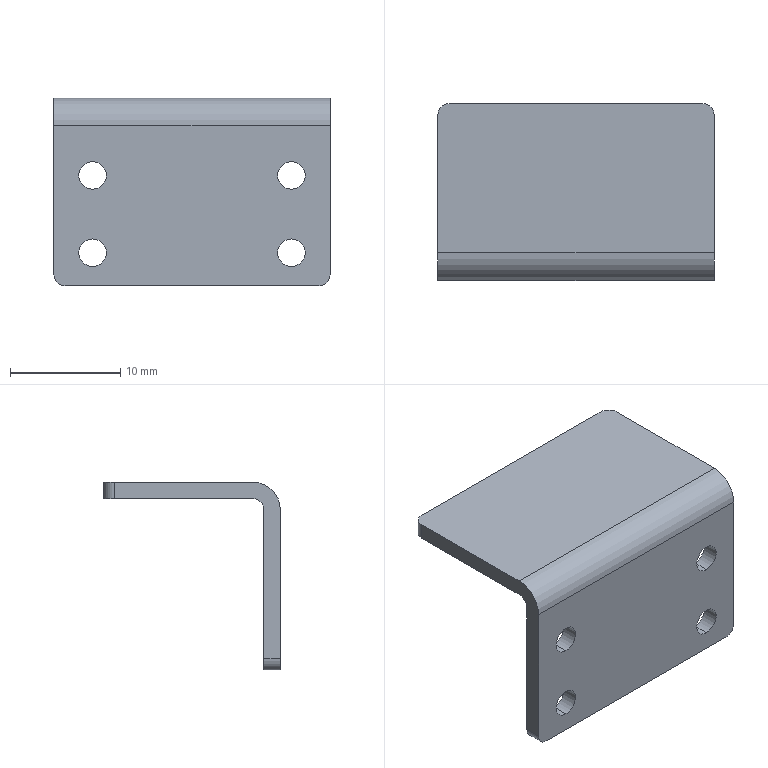Part | SolidWorks | features BaseBody 1 | 1 solid | 22 faces | box 25 x 16 x 17 mm | volume 1122 mm3 | cylinder 14 | plane 8 | commonest cylinder face diameters 2.5 x8 2 x5 5 x1
STEP:
#1=CARTESIAN_POINT('',(100.5,20.,-73.25));
#2=VERTEX_POINT('',#1);
#3=CARTESIAN_POINT('',(100.5,20.,-75.75));
#4=VERTEX_POINT('',#3);
#5=CARTESIAN_POINT('',(100.5,20.,-74.5));
#6=DIRECTION('',(0.,-1.,0.));
#7=DIRECTION('',(0.,0.,1.));
#8=AXIS2_PLACEMENT_3D('',#5,#6,#7);
#9=CIRCLE('',#8,1.25);
#10=EDGE_CURVE('',#2,#4,#9,.T.);
#11=ORIENTED_EDGE('',*,*,#10,.T.);
#12=CARTESIAN_POINT('',(100.5,21.5,-75.75));
#13=VERTEX_POINT('',#12);
#14=CARTESIAN_POINT('',(100.5,46.5,-75.75));
#15=DIRECTION('',(0.,1.,0.));
#16=VECTOR('',#15,1000.);
#17=LINE('',#14,#16);
#18=EDGE_CURVE('',#4,#13,#17,.T.);
#19=ORIENTED_EDGE('',*,*,#18,.T.);
#20=CARTESIAN_POINT('',(100.5,21.5,-73.25));
#21=VERTEX_POINT('',#20);
#22=CARTESIAN_POINT('',(100.5,21.5,-74.5));
#23=DIRECTION('',(0.,-1.,0.));
#24=DIRECTION('',(0.,0.,1.));
#25=AXIS2_PLACEMENT_3D('',#22,#23,#24);
#26=CIRCLE('',#25,1.25);
#27=EDGE_CURVE('',#21,#13,#26,.T.);
#28=ORIENTED_EDGE('',*,*,#27,.F.);
#29=CARTESIAN_POINT('',(100.5,46.5,-73.25));
#30=DIRECTION('',(0.,1.,0.));
#31=VECTOR('',#30,1000.);
#32=LINE('',#29,#31);
#33=EDGE_CURVE('',#2,#21,#32,.T.);
#34=ORIENTED_EDGE('',*,*,#33,.F.);
#35=EDGE_LOOP('',(#11,#19,#28,#34));
#36=FACE_OUTER_BOUND('',#35,.T.);
#37=CARTESIAN_POINT('',(100.5,46.5,-74.5));
#38=DIRECTION('',(0.,1.,0.));
#39=DIRECTION('',(0.,0.,1.));
#40=AXIS2_PLACEMENT_3D('',#37,#38,#39);
#41=CYLINDRICAL_SURFACE('',#40,1.25);
#42=ADVANCED_FACE('',(#36),#41,.F.);
#43=CARTESIAN_POINT('',(118.5,20.,-80.25));
#44=VERTEX_POINT('',#43);
#45=CARTESIAN_POINT('',(118.5,20.,-82.75));
#46=VERTEX_POINT('',#45);
#47=CARTESIAN_POINT('',(118.5,20.,-81.5));
#48=DIRECTION('',(0.,-1.,0.));
#49=DIRECTION('',(0.,0.,1.));
#50=AXIS2_PLACEMENT_3D('',#47,#48,#49);
#51=CIRCLE('',#50,1.25);
#52=EDGE_CURVE('',#44,#46,#51,.T.);
#53=ORIENTED_EDGE('',*,*,#52,.T.);
#54=CARTESIAN_POINT('',(118.5,21.5,-82.75));
#55=VERTEX_POINT('',#54);
#56=CARTESIAN_POINT('',(118.5,46.5,-82.75));
#57=DIRECTION('',(0.,1.,0.));
#58=VECTOR('',#57,1000.);
#59=LINE('',#56,#58);
#60=EDGE_CURVE('',#46,#55,#59,.T.);
#61=ORIENTED_EDGE('',*,*,#60,.T.);
#62=CARTESIAN_POINT('',(118.5,21.5,-80.25));
#63=VERTEX_POINT('',#62);
#64=CARTESIAN_POINT('',(118.5,21.5,-81.5));
#65=DIRECTION('',(0.,-1.,0.));
#66=DIRECTION('',(0.,0.,1.));
#67=AXIS2_PLACEMENT_3D('',#64,#65,#66);
#68=CIRCLE('',#67,1.25);
#69=EDGE_CURVE('',#63,#55,#68,.T.);
#70=ORIENTED_EDGE('',*,*,#69,.F.);
#71=CARTESIAN_POINT('',(118.5,46.5,-80.25));
#72=DIRECTION('',(0.,1.,0.));
#73=VECTOR('',#72,1000.);
#74=LINE('',#71,#73);
#75=EDGE_CURVE('',#44,#63,#74,.T.);
#76=ORIENTED_EDGE('',*,*,#75,.F.);
#77=EDGE_LOOP('',(#53,#61,#70,#76));
#78=FACE_OUTER_BOUND('',#77,.T.);
#79=CARTESIAN_POINT('',(118.5,46.5,-81.5));
#80=DIRECTION('',(0.,1.,0.));
#81=DIRECTION('',(0.,0.,1.));
#82=AXIS2_PLACEMENT_3D('',#79,#80,#81);
#83=CYLINDRICAL_SURFACE('',#82,1.25);
#84=ADVANCED_FACE('',(#78),#83,.F.);
#85=CARTESIAN_POINT('',(100.5,20.,-80.25));
#86=VERTEX_POINT('',#85);
#87=CARTESIAN_POINT('',(100.5,20.,-82.75));
#88=VERTEX_POINT('',#87);
#89=CARTESIAN_POINT('',(100.5,20.,-81.5));
#90=DIRECTION('',(0.,-1.,0.));
#91=DIRECTION('',(0.,0.,1.));
#92=AXIS2_PLACEMENT_3D('',#89,#90,#91);
#93=CIRCLE('',#92,1.25);
#94=EDGE_CURVE('',#86,#88,#93,.T.);
#95=ORIENTED_EDGE('',*,*,#94,.T.);
#96=CARTESIAN_POINT('',(100.5,21.5,-82.75));
#97=VERTEX_POINT('',#96);
#98=CARTESIAN_POINT('',(100.5,46.5,-82.75));
#99=DIRECTION('',(0.,1.,0.));
#100=VECTOR('',#99,1000.);
#101=LINE('',#98,#100);
#102=EDGE_CURVE('',#88,#97,#101,.T.);
#103=ORIENTED_EDGE('',*,*,#102,.T.);
#104=CARTESIAN_POINT('',(100.5,21.5,-80.25));
#105=VERTEX_POINT('',#104);
#106=CARTESIAN_POINT('',(100.5,21.5,-81.5));
#107=DIRECTION('',(0.,-1.,0.));
#108=DIRECTION('',(0.,0.,1.));
#109=AXIS2_PLACEMENT_3D('',#106,#107,#108);
#110=CIRCLE('',#109,1.25);
#111=EDGE_CURVE('',#105,#97,#110,.T.);
#112=ORIENTED_EDGE('',*,*,#111,.F.);
#113=CARTESIAN_POINT('',(100.5,46.5,-80.25));
#114=DIRECTION('',(0.,1.,0.));
#115=VECTOR('',#114,1000.);
#116=LINE('',#113,#115);
#117=EDGE_CURVE('',#86,#105,#116,.T.);
#118=ORIENTED_EDGE('',*,*,#117,.F.);
#119=EDGE_LOOP('',(#95,#103,#112,#118));
#120=FACE_OUTER_BOUND('',#119,.T.);
#121=CARTESIAN_POINT('',(100.5,46.5,-81.5));
#122=DIRECTION('',(0.,1.,0.));
#123=DIRECTION('',(0.,0.,1.));
#124=AXIS2_PLACEMENT_3D('',#121,#122,#123);
#125=CYLINDRICAL_SURFACE('',#124,1.25);
#126=ADVANCED_FACE('',(#120),#125,.F.);
#127=CARTESIAN_POINT('',(118.5,20.,-73.25));
#128=VERTEX_POINT('',#127);
#129=CARTESIAN_POINT('',(118.5,20.,-75.75));
#130=VERTEX_POINT('',#129);
#131=CARTESIAN_POINT('',(118.5,20.,-74.5));
#132=DIRECTION('',(0.,-1.,0.));
#133=DIRECTION('',(0.,0.,1.));
#134=AXIS2_PLACEMENT_3D('',#131,#132,#133);
#135=CIRCLE('',#134,1.25);
#136=EDGE_CURVE('',#128,#130,#135,.T.);
#137=ORIENTED_EDGE('',*,*,#136,.T.);
#138=CARTESIAN_POINT('',(118.5,21.5,-75.75));
#139=VERTEX_POINT('',#138);
#140=CARTESIAN_POINT('',(118.5,46.5,-75.75));
#141=DIRECTION('',(0.,1.,0.));
#142=VECTOR('',#141,1000.);
#143=LINE('',#140,#142);
#144=EDGE_CURVE('',#130,#139,#143,.T.);
#145=ORIENTED_EDGE('',*,*,#144,.T.);
#146=CARTESIAN_POINT('',(118.5,21.5,-73.25));
#147=VERTEX_POINT('',#146);
#148=CARTESIAN_POINT('',(118.5,21.5,-74.5));
#149=DIRECTION('',(0.,-1.,0.));
#150=DIRECTION('',(0.,0.,1.));
#151=AXIS2_PLACEMENT_3D('',#148,#149,#150);
#152=CIRCLE('',#151,1.25);
#153=EDGE_CURVE('',#147,#139,#152,.T.);
#154=ORIENTED_EDGE('',*,*,#153,.F.);
#155=CARTESIAN_POINT('',(118.5,46.5,-73.25));
#156=DIRECTION('',(0.,1.,0.));
#157=VECTOR('',#156,1000.);
#158=LINE('',#155,#157);
#159=EDGE_CURVE('',#128,#147,#158,.T.);
#160=ORIENTED_EDGE('',*,*,#159,.F.);
#161=EDGE_LOOP('',(#137,#145,#154,#160));
#162=FACE_OUTER_BOUND('',#161,.T.);
#163=CARTESIAN_POINT('',(118.5,46.5,-74.5));
#164=DIRECTION('',(0.,1.,0.));
#165=DIRECTION('',(0.,0.,1.));
#166=AXIS2_PLACEMENT_3D('',#163,#164,#165);
#167=CYLINDRICAL_SURFACE('',#166,1.25);
#168=ADVANCED_FACE('',(#162),#167,.F.);
#169=CARTESIAN_POINT('',(122.,20.,-83.5));
#170=VERTEX_POINT('',#169);
#171=CARTESIAN_POINT('',(121.,20.,-84.5));
#172=VERTEX_POINT('',#171);
#173=CARTESIAN_POINT('',(121.,20.,-83.5));
#174=DIRECTION('',(0.,1.,0.));
#175=DIRECTION('',(0.,0.,1.));
#176=AXIS2_PLACEMENT_3D('',#173,#174,#175);
#177=CIRCLE('',#176,1.);
#178=EDGE_CURVE('',#170,#172,#177,.T.);
#179=ORIENTED_EDGE('',*,*,#178,.F.);
#180=CARTESIAN_POINT('',(122.,20.,-70.));
#181=VERTEX_POINT('',#180);
#182=CARTESIAN_POINT('',(122.,20.,-70.));
#183=DIRECTION('',(0.,0.,-1.));
#184=VECTOR('',#183,1000.);
#185=LINE('',#182,#184);
#186=EDGE_CURVE('',#181,#170,#185,.T.);
#187=ORIENTED_EDGE('',*,*,#186,.F.);
#188=CARTESIAN_POINT('',(97.,20.,-70.));
#189=VERTEX_POINT('',#188);
#190=CARTESIAN_POINT('',(122.,20.,-70.));
#191=DIRECTION('',(1.,0.,0.));
#192=VECTOR('',#191,1000.);
#193=LINE('',#190,#192);
#194=EDGE_CURVE('',#189,#181,#193,.T.);
#195=ORIENTED_EDGE('',*,*,#194,.F.);
#196=CARTESIAN_POINT('',(97.,20.,-83.5));
#197=VERTEX_POINT('',#196);
#198=CARTESIAN_POINT('',(97.,20.,-70.));
#199=DIRECTION('',(0.,0.,1.));
#200=VECTOR('',#199,1000.);
#201=LINE('',#198,#200);
#202=EDGE_CURVE('',#197,#189,#201,.T.);
#203=ORIENTED_EDGE('',*,*,#202,.F.);
#204=CARTESIAN_POINT('',(98.,20.,-84.5));
#205=VERTEX_POINT('',#204);
#206=CARTESIAN_POINT('',(98.,20.,-83.5));
#207=DIRECTION('',(0.,1.,0.));
#208=DIRECTION('',(0.,0.,-1.));
#209=AXIS2_PLACEMENT_3D('',#206,#207,#208);
#210=CIRCLE('',#209,1.);
#211=EDGE_CURVE('',#205,#197,#210,.T.);
#212=ORIENTED_EDGE('',*,*,#211,.F.);
#213=CARTESIAN_POINT('',(122.,20.,-84.5));
#214=DIRECTION('',(-1.,0.,0.));
#215=VECTOR('',#214,1000.);
#216=LINE('',#213,#215);
#217=EDGE_CURVE('',#172,#205,#216,.T.);
#218=ORIENTED_EDGE('',*,*,#217,.F.);
#219=EDGE_LOOP('',(#179,#187,#195,#203,#212,#218));
#220=FACE_OUTER_BOUND('',#219,.T.);
#221=ORIENTED_EDGE('',*,*,#10,.F.);
#222=CARTESIAN_POINT('',(100.5,20.,-74.5));
#223=DIRECTION('',(0.,-1.,0.));
#224=DIRECTION('',(0.,0.,1.));
#225=AXIS2_PLACEMENT_3D('',#222,#223,#224);
#226=CIRCLE('',#225,1.25);
#227=EDGE_CURVE('',#4,#2,#226,.T.);
#228=ORIENTED_EDGE('',*,*,#227,.F.);
#229=EDGE_LOOP('',(#221,#228));
#230=FACE_BOUND('',#229,.T.);
#231=ORIENTED_EDGE('',*,*,#52,.F.);
#232=CARTESIAN_POINT('',(118.5,20.,-81.5));
#233=DIRECTION('',(0.,-1.,0.));
#234=DIRECTION('',(0.,0.,1.));
#235=AXIS2_PLACEMENT_3D('',#232,#233,#234);
#236=CIRCLE('',#235,1.25);
#237=EDGE_CURVE('',#46,#44,#236,.T.);
#238=ORIENTED_EDGE('',*,*,#237,.F.);
#239=EDGE_LOOP('',(#231,#238));
#240=FACE_BOUND('',#239,.T.);
#241=ORIENTED_EDGE('',*,*,#94,.F.);
#242=CARTESIAN_POINT('',(100.5,20.,-81.5));
#243=DIRECTION('',(0.,-1.,0.));
#244=DIRECTION('',(0.,0.,1.));
#245=AXIS2_PLACEMENT_3D('',#242,#243,#244);
#246=CIRCLE('',#245,1.25);
#247=EDGE_CURVE('',#88,#86,#246,.T.);
#248=ORIENTED_EDGE('',*,*,#247,.F.);
#249=EDGE_LOOP('',(#241,#248));
#250=FACE_BOUND('',#249,.T.);
#251=ORIENTED_EDGE('',*,*,#136,.F.);
#252=CARTESIAN_POINT('',(118.5,20.,-74.5));
#253=DIRECTION('',(0.,-1.,0.));
#254=DIRECTION('',(0.,0.,1.));
#255=AXIS2_PLACEMENT_3D('',#252,#253,#254);
#256=CIRCLE('',#255,1.25);
#257=EDGE_CURVE('',#130,#128,#256,.T.);
#258=ORIENTED_EDGE('',*,*,#257,.F.);
#259=EDGE_LOOP('',(#251,#258));
#260=FACE_BOUND('',#259,.T.);
#261=CARTESIAN_POINT('',(122.,20.,-70.));
#262=DIRECTION('',(0.,1.,0.));
#263=DIRECTION('',(0.,0.,1.));
#264=AXIS2_PLACEMENT_3D('',#261,#262,#263);
#265=PLANE('',#264);
#266=ADVANCED_FACE('',(#220,#230,#240,#250,#260),#265,.F.);
#267=CARTESIAN_POINT('',(121.,21.5,-84.5));
#268=VERTEX_POINT('',#267);
#269=CARTESIAN_POINT('',(121.,20.,-84.5));
#270=DIRECTION('',(0.,1.,0.));
#271=VECTOR('',#270,1000.);
#272=LINE('',#269,#271);
#273=EDGE_CURVE('',#172,#268,#272,.T.);
#274=ORIENTED_EDGE('',*,*,#273,.F.);
#275=ORIENTED_EDGE('',*,*,#217,.T.);
#276=CARTESIAN_POINT('',(98.,21.5,-84.5));
#277=VERTEX_POINT('',#276);
#278=CARTESIAN_POINT('',(98.,20.,-84.5));
#279=DIRECTION('',(0.,-1.,0.));
#280=VECTOR('',#279,1000.);
#281=LINE('',#278,#280);
#282=EDGE_CURVE('',#277,#205,#281,.T.);
#283=ORIENTED_EDGE('',*,*,#282,.F.);
#284=CARTESIAN_POINT('',(122.,21.5,-84.5));
#285=DIRECTION('',(-1.,0.,0.));
#286=VECTOR('',#285,1000.);
#287=LINE('',#284,#286);
#288=EDGE_CURVE('',#268,#277,#287,.T.);
#289=ORIENTED_EDGE('',*,*,#288,.F.);
#290=EDGE_LOOP('',(#274,#275,#283,#289));
#291=FACE_OUTER_BOUND('',#290,.T.);
#292=CARTESIAN_POINT('',(122.,20.,-84.5));
#293=DIRECTION('',(0.,0.,1.));
#294=DIRECTION('',(1.,0.,0.));
#295=AXIS2_PLACEMENT_3D('',#292,#293,#294);
#296=PLANE('',#295);
#297=ADVANCED_FACE('',(#291),#296,.F.);
#298=CARTESIAN_POINT('',(122.,21.5,-83.5));
#299=VERTEX_POINT('',#298);
#300=CARTESIAN_POINT('',(121.,21.5,-83.5));
#301=DIRECTION('',(0.,-1.,0.));
#302=DIRECTION('',(0.,0.,1.));
#303=AXIS2_PLACEMENT_3D('',#300,#301,#302);
#304=CIRCLE('',#303,1.);
#305=EDGE_CURVE('',#268,#299,#304,.T.);
#306=ORIENTED_EDGE('',*,*,#305,.T.);
#307=CARTESIAN_POINT('',(122.,22.5,-83.5));
#308=DIRECTION('',(0.,-1.,0.));
#309=VECTOR('',#308,1000.);
#310=LINE('',#307,#309);
#311=EDGE_CURVE('',#299,#170,#310,.T.);
#312=ORIENTED_EDGE('',*,*,#311,.T.);
#313=ORIENTED_EDGE('',*,*,#178,.T.);
#314=ORIENTED_EDGE('',*,*,#273,.T.);
#315=EDGE_LOOP('',(#306,#312,#313,#314));
#316=FACE_OUTER_BOUND('',#315,.T.);
#317=CARTESIAN_POINT('',(121.,22.5,-83.5));
#318=DIRECTION('',(0.,1.,0.));
#319=DIRECTION('',(0.,0.,1.));
#320=AXIS2_PLACEMENT_3D('',#317,#318,#319);
#321=CYLINDRICAL_SURFACE('',#320,1.);
#322=ADVANCED_FACE('',(#316),#321,.T.);
#323=CARTESIAN_POINT('',(122.,35.,-67.5));
#324=VERTEX_POINT('',#323);
#325=CARTESIAN_POINT('',(122.,22.5,-67.5));
#326=VERTEX_POINT('',#325);
#327=CARTESIAN_POINT('',(122.,22.5,-67.5));
#328=DIRECTION('',(0.,-1.,0.));
#329=VECTOR('',#328,1000.);
#330=LINE('',#327,#329);
#331=EDGE_CURVE('',#324,#326,#330,.T.);
#332=ORIENTED_EDGE('',*,*,#331,.T.);
#333=CARTESIAN_POINT('',(122.,22.5,-70.));
#334=DIRECTION('',(1.,0.,0.));
#335=DIRECTION('',(0.,0.,-1.));
#336=AXIS2_PLACEMENT_3D('',#333,#334,#335);
#337=CIRCLE('',#336,2.5);
#338=EDGE_CURVE('',#326,#181,#337,.T.);
#339=ORIENTED_EDGE('',*,*,#338,.T.);
#340=ORIENTED_EDGE('',*,*,#186,.T.);
#341=ORIENTED_EDGE('',*,*,#311,.F.);
#342=CARTESIAN_POINT('',(122.,21.5,-70.));
#343=VERTEX_POINT('',#342);
#344=CARTESIAN_POINT('',(122.,21.5,-70.));
#345=DIRECTION('',(0.,0.,1.));
#346=VECTOR('',#345,1000.);
#347=LINE('',#344,#346);
#348=EDGE_CURVE('',#299,#343,#347,.T.);
#349=ORIENTED_EDGE('',*,*,#348,.T.);
#350=CARTESIAN_POINT('',(122.,22.5,-69.));
#351=VERTEX_POINT('',#350);
#352=CARTESIAN_POINT('',(122.,22.5,-70.));
#353=DIRECTION('',(-1.,0.,0.));
#354=DIRECTION('',(0.,0.,-1.));
#355=AXIS2_PLACEMENT_3D('',#352,#353,#354);
#356=CIRCLE('',#355,1.);
#357=EDGE_CURVE('',#343,#351,#356,.T.);
#358=ORIENTED_EDGE('',*,*,#357,.T.);
#359=CARTESIAN_POINT('',(122.,35.,-69.));
#360=VERTEX_POINT('',#359);
#361=CARTESIAN_POINT('',(122.,22.5,-69.));
#362=DIRECTION('',(0.,1.,0.));
#363=VECTOR('',#362,1000.);
#364=LINE('',#361,#363);
#365=EDGE_CURVE('',#351,#360,#364,.T.);
#366=ORIENTED_EDGE('',*,*,#365,.T.);
#367=CARTESIAN_POINT('',(122.,35.,-70.));
#368=DIRECTION('',(0.,0.,1.));
#369=VECTOR('',#368,1000.);
#370=LINE('',#367,#369);
#371=EDGE_CURVE('',#360,#324,#370,.T.);
#372=ORIENTED_EDGE('',*,*,#371,.T.);
#373=EDGE_LOOP('',(#332,#339,#340,#341,#349,#358,#366,#372));
#374=FACE_OUTER_BOUND('',#373,.T.);
#375=CARTESIAN_POINT('',(122.,22.5,-70.));
#376=DIRECTION('',(1.,0.,0.));
#377=DIRECTION('',(0.,0.,-1.));
#378=AXIS2_PLACEMENT_3D('',#375,#376,#377);
#379=PLANE('',#378);
#380=ADVANCED_FACE('',(#374),#379,.T.);
#381=ORIENTED_EDGE('',*,*,#338,.F.);
#382=CARTESIAN_POINT('',(97.,22.5,-67.5));
#383=VERTEX_POINT('',#382);
#384=CARTESIAN_POINT('',(122.,22.5,-67.5));
#385=DIRECTION('',(-1.,0.,0.));
#386=VECTOR('',#385,1000.);
#387=LINE('',#384,#386);
#388=EDGE_CURVE('',#326,#383,#387,.T.);
#389=ORIENTED_EDGE('',*,*,#388,.T.);
#390=CARTESIAN_POINT('',(97.,22.5,-70.));
#391=DIRECTION('',(1.,0.,0.));
#392=DIRECTION('',(0.,0.,-1.));
#393=AXIS2_PLACEMENT_3D('',#390,#391,#392);
#394=CIRCLE('',#393,2.5);
#395=EDGE_CURVE('',#383,#189,#394,.T.);
#396=ORIENTED_EDGE('',*,*,#395,.T.);
#397=ORIENTED_EDGE('',*,*,#194,.T.);
#398=EDGE_LOOP('',(#381,#389,#396,#397));
#399=FACE_OUTER_BOUND('',#398,.T.);
#400=CARTESIAN_POINT('',(122.,22.5,-70.));
#401=DIRECTION('',(1.,0.,0.));
#402=DIRECTION('',(0.,0.,-1.));
#403=AXIS2_PLACEMENT_3D('',#400,#401,#402);
#404=CYLINDRICAL_SURFACE('',#403,2.5);
#405=ADVANCED_FACE('',(#399),#404,.T.);
#406=CARTESIAN_POINT('',(97.,21.5,-83.5));
#407=VERTEX_POINT('',#406);
#408=CARTESIAN_POINT('',(97.,22.5,-83.5));
#409=DIRECTION('',(0.,1.,0.));
#410=VECTOR('',#409,1000.);
#411=LINE('',#408,#410);
#412=EDGE_CURVE('',#197,#407,#411,.T.);
#413=ORIENTED_EDGE('',*,*,#412,.F.);
#414=ORIENTED_EDGE('',*,*,#202,.T.);
#415=ORIENTED_EDGE('',*,*,#395,.F.);
#416=CARTESIAN_POINT('',(97.,35.,-67.5));
#417=VERTEX_POINT('',#416);
#418=CARTESIAN_POINT('',(97.,22.5,-67.5));
#419=DIRECTION('',(0.,-1.,0.));
#420=VECTOR('',#419,1000.);
#421=LINE('',#418,#420);
#422=EDGE_CURVE('',#417,#383,#421,.T.);
#423=ORIENTED_EDGE('',*,*,#422,.F.);
#424=CARTESIAN_POINT('',(97.,35.,-69.));
#425=VERTEX_POINT('',#424);
#426=CARTESIAN_POINT('',(97.,35.,-70.));
#427=DIRECTION('',(0.,0.,1.));
#428=VECTOR('',#427,1000.);
#429=LINE('',#426,#428);
#430=EDGE_CURVE('',#425,#417,#429,.T.);
#431=ORIENTED_EDGE('',*,*,#430,.F.);
#432=CARTESIAN_POINT('',(97.,22.5,-69.));
#433=VERTEX_POINT('',#432);
#434=CARTESIAN_POINT('',(97.,22.5,-69.));
#435=DIRECTION('',(0.,1.,0.));
#436=VECTOR('',#435,1000.);
#437=LINE('',#434,#436);
#438=EDGE_CURVE('',#433,#425,#437,.T.);
#439=ORIENTED_EDGE('',*,*,#438,.F.);
#440=CARTESIAN_POINT('',(97.,21.5,-70.));
#441=VERTEX_POINT('',#440);
#442=CARTESIAN_POINT('',(97.,22.5,-70.));
#443=DIRECTION('',(1.,0.,0.));
#444=DIRECTION('',(0.,0.,-1.));
#445=AXIS2_PLACEMENT_3D('',#442,#443,#444);
#446=CIRCLE('',#445,1.);
#447=EDGE_CURVE('',#433,#441,#446,.T.);
#448=ORIENTED_EDGE('',*,*,#447,.T.);
#449=CARTESIAN_POINT('',(97.,21.5,-70.));
#450=DIRECTION('',(0.,0.,1.));
#451=VECTOR('',#450,1000.);
#452=LINE('',#449,#451);
#453=EDGE_CURVE('',#407,#441,#452,.T.);
#454=ORIENTED_EDGE('',*,*,#453,.F.);
#455=EDGE_LOOP('',(#413,#414,#415,#423,#431,#439,#448,#454));
#456=FACE_OUTER_BOUND('',#455,.T.);
#457=CARTESIAN_POINT('',(97.,22.5,-70.));
#458=DIRECTION('',(1.,0.,0.));
#459=DIRECTION('',(0.,0.,-1.));
#460=AXIS2_PLACEMENT_3D('',#457,#458,#459);
#461=PLANE('',#460);
#462=ADVANCED_FACE('',(#456),#461,.F.);
#463=CARTESIAN_POINT('',(98.,21.5,-83.5));
#464=DIRECTION('',(0.,-1.,0.));
#465=DIRECTION('',(0.,0.,-1.));
#466=AXIS2_PLACEMENT_3D('',#463,#464,#465);
#467=CIRCLE('',#466,1.);
#468=EDGE_CURVE('',#407,#277,#467,.T.);
#469=ORIENTED_EDGE('',*,*,#468,.T.);
#470=ORIENTED_EDGE('',*,*,#282,.T.);
#471=ORIENTED_EDGE('',*,*,#211,.T.);
#472=ORIENTED_EDGE('',*,*,#412,.T.);
#473=EDGE_LOOP('',(#469,#470,#471,#472));
#474=FACE_OUTER_BOUND('',#473,.T.);
#475=CARTESIAN_POINT('',(98.,20.,-83.5));
#476=DIRECTION('',(0.,-1.,0.));
#477=DIRECTION('',(0.,0.,-1.));
#478=AXIS2_PLACEMENT_3D('',#475,#476,#477);
#479=CYLINDRICAL_SURFACE('',#478,1.);
#480=ADVANCED_FACE('',(#474),#479,.T.);
#481=ORIENTED_EDGE('',*,*,#18,.F.);
#482=ORIENTED_EDGE('',*,*,#227,.T.);
#483=ORIENTED_EDGE('',*,*,#33,.T.);
#484=CARTESIAN_POINT('',(100.5,21.5,-74.5));
#485=DIRECTION('',(0.,-1.,0.));
#486=DIRECTION('',(0.,0.,1.));
#487=AXIS2_PLACEMENT_3D('',#484,#485,#486);
#488=CIRCLE('',#487,1.25);
#489=EDGE_CURVE('',#13,#21,#488,.T.);
#490=ORIENTED_EDGE('',*,*,#489,.F.);
#491=EDGE_LOOP('',(#481,#482,#483,#490));
#492=FACE_OUTER_BOUND('',#491,.T.);
#493=CARTESIAN_POINT('',(100.5,46.5,-74.5));
#494=DIRECTION('',(0.,1.,0.));
#495=DIRECTION('',(0.,0.,1.));
#496=AXIS2_PLACEMENT_3D('',#493,#494,#495);
#497=CYLINDRICAL_SURFACE('',#496,1.25);
#498=ADVANCED_FACE('',(#492),#497,.F.);
#499=ORIENTED_EDGE('',*,*,#60,.F.);
#500=ORIENTED_EDGE('',*,*,#237,.T.);
#501=ORIENTED_EDGE('',*,*,#75,.T.);
#502=CARTESIAN_POINT('',(118.5,21.5,-81.5));
#503=DIRECTION('',(0.,-1.,0.));
#504=DIRECTION('',(0.,0.,1.));
#505=AXIS2_PLACEMENT_3D('',#502,#503,#504);
#506=CIRCLE('',#505,1.25);
#507=EDGE_CURVE('',#55,#63,#506,.T.);
#508=ORIENTED_EDGE('',*,*,#507,.F.);
#509=EDGE_LOOP('',(#499,#500,#501,#508));
#510=FACE_OUTER_BOUND('',#509,.T.);
#511=CARTESIAN_POINT('',(118.5,46.5,-81.5));
#512=DIRECTION('',(0.,1.,0.));
#513=DIRECTION('',(0.,0.,1.));
#514=AXIS2_PLACEMENT_3D('',#511,#512,#513);
#515=CYLINDRICAL_SURFACE('',#514,1.25);
#516=ADVANCED_FACE('',(#510),#515,.F.);
#517=ORIENTED_EDGE('',*,*,#102,.F.);
#518=ORIENTED_EDGE('',*,*,#247,.T.);
#519=ORIENTED_EDGE('',*,*,#117,.T.);
#520=CARTESIAN_POINT('',(100.5,21.5,-81.5));
#521=DIRECTION('',(0.,-1.,0.));
#522=DIRECTION('',(0.,0.,1.));
#523=AXIS2_PLACEMENT_3D('',#520,#521,#522);
#524=CIRCLE('',#523,1.25);
#525=EDGE_CURVE('',#97,#105,#524,.T.);
#526=ORIENTED_EDGE('',*,*,#525,.F.);
#527=EDGE_LOOP('',(#517,#518,#519,#526));
#528=FACE_OUTER_BOUND('',#527,.T.);
#529=CARTESIAN_POINT('',(100.5,46.5,-81.5));
#530=DIRECTION('',(0.,1.,0.));
#531=DIRECTION('',(0.,0.,1.));
#532=AXIS2_PLACEMENT_3D('',#529,#530,#531);
#533=CYLINDRICAL_SURFACE('',#532,1.25);
#534=ADVANCED_FACE('',(#528),#533,.F.);
#535=ORIENTED_EDGE('',*,*,#144,.F.);
#536=ORIENTED_EDGE('',*,*,#257,.T.);
#537=ORIENTED_EDGE('',*,*,#159,.T.);
#538=CARTESIAN_POINT('',(118.5,21.5,-74.5));
#539=DIRECTION('',(0.,-1.,0.));
#540=DIRECTION('',(0.,0.,1.));
#541=AXIS2_PLACEMENT_3D('',#538,#539,#540);
#542=CIRCLE('',#541,1.25);
#543=EDGE_CURVE('',#139,#147,#542,.T.);
#544=ORIENTED_EDGE('',*,*,#543,.F.);
#545=EDGE_LOOP('',(#535,#536,#537,#544));
#546=FACE_OUTER_BOUND('',#545,.T.);
#547=CARTESIAN_POINT('',(118.5,46.5,-74.5));
#548=DIRECTION('',(0.,1.,0.));
#549=DIRECTION('',(0.,0.,1.));
#550=AXIS2_PLACEMENT_3D('',#547,#548,#549);
#551=CYLINDRICAL_SURFACE('',#550,1.25);
#552=ADVANCED_FACE('',(#546),#551,.F.);
#553=ORIENTED_EDGE('',*,*,#305,.F.);
#554=ORIENTED_EDGE('',*,*,#288,.T.);
#555=ORIENTED_EDGE('',*,*,#468,.F.);
#556=ORIENTED_EDGE('',*,*,#453,.T.);
#557=CARTESIAN_POINT('',(122.,21.5,-70.));
#558=DIRECTION('',(-1.,0.,0.));
#559=VECTOR('',#558,1000.);
#560=LINE('',#557,#559);
#561=EDGE_CURVE('',#343,#441,#560,.T.);
#562=ORIENTED_EDGE('',*,*,#561,.F.);
#563=ORIENTED_EDGE('',*,*,#348,.F.);
#564=EDGE_LOOP('',(#553,#554,#555,#556,#562,#563));
#565=FACE_OUTER_BOUND('',#564,.T.);
#566=ORIENTED_EDGE('',*,*,#27,.T.);
#567=ORIENTED_EDGE('',*,*,#489,.T.);
#568=EDGE_LOOP('',(#566,#567));
#569=FACE_BOUND('',#568,.T.);
#570=ORIENTED_EDGE('',*,*,#69,.T.);
#571=ORIENTED_EDGE('',*,*,#507,.T.);
#572=EDGE_LOOP('',(#570,#571));
#573=FACE_BOUND('',#572,.T.);
#574=ORIENTED_EDGE('',*,*,#111,.T.);
#575=ORIENTED_EDGE('',*,*,#525,.T.);
#576=EDGE_LOOP('',(#574,#575));
#577=FACE_BOUND('',#576,.T.);
#578=ORIENTED_EDGE('',*,*,#153,.T.);
#579=ORIENTED_EDGE('',*,*,#543,.T.);
#580=EDGE_LOOP('',(#578,#579));
#581=FACE_BOUND('',#580,.T.);
#582=CARTESIAN_POINT('',(122.,21.5,-84.5));
#583=DIRECTION('',(0.,-1.,0.));
#584=DIRECTION('',(0.,0.,-1.));
#585=AXIS2_PLACEMENT_3D('',#582,#583,#584);
#586=PLANE('',#585);
#587=ADVANCED_FACE('',(#565,#569,#573,#577,#581),#586,.F.);
#588=CARTESIAN_POINT('',(121.,36.,-67.5));
#589=VERTEX_POINT('',#588);
#590=CARTESIAN_POINT('',(121.,35.,-67.5));
#591=DIRECTION('',(0.,0.,-1.));
#592=DIRECTION('',(1.,0.,0.));
#593=AXIS2_PLACEMENT_3D('',#590,#591,#592);
#594=CIRCLE('',#593,1.);
#595=EDGE_CURVE('',#589,#324,#594,.T.);
#596=ORIENTED_EDGE('',*,*,#595,.F.);
#597=CARTESIAN_POINT('',(98.,36.,-67.5));
#598=VERTEX_POINT('',#597);
#599=CARTESIAN_POINT('',(122.,36.,-67.5));
#600=DIRECTION('',(1.,0.,0.));
#601=VECTOR('',#600,1000.);
#602=LINE('',#599,#601);
#603=EDGE_CURVE('',#598,#589,#602,.T.);
#604=ORIENTED_EDGE('',*,*,#603,.F.);
#605=CARTESIAN_POINT('',(98.,35.,-67.5));
#606=DIRECTION('',(0.,0.,-1.));
#607=DIRECTION('',(-1.,0.,0.));
#608=AXIS2_PLACEMENT_3D('',#605,#606,#607);
#609=CIRCLE('',#608,1.);
#610=EDGE_CURVE('',#417,#598,#609,.T.);
#611=ORIENTED_EDGE('',*,*,#610,.F.);
#612=ORIENTED_EDGE('',*,*,#422,.T.);
#613=ORIENTED_EDGE('',*,*,#388,.F.);
#614=ORIENTED_EDGE('',*,*,#331,.F.);
#615=EDGE_LOOP('',(#596,#604,#611,#612,#613,#614));
#616=FACE_OUTER_BOUND('',#615,.T.);
#617=CARTESIAN_POINT('',(122.,36.,-67.5));
#618=DIRECTION('',(0.,0.,-1.));
#619=DIRECTION('',(-1.,0.,0.));
#620=AXIS2_PLACEMENT_3D('',#617,#618,#619);
#621=PLANE('',#620);
#622=ADVANCED_FACE('',(#616),#621,.F.);
#623=ORIENTED_EDGE('',*,*,#595,.T.);
#624=ORIENTED_EDGE('',*,*,#371,.F.);
#625=CARTESIAN_POINT('',(121.,36.,-69.));
#626=VERTEX_POINT('',#625);
#627=CARTESIAN_POINT('',(121.,35.,-69.));
#628=DIRECTION('',(0.,0.,1.));
#629=DIRECTION('',(1.,0.,0.));
#630=AXIS2_PLACEMENT_3D('',#627,#628,#629);
#631=CIRCLE('',#630,1.);
#632=EDGE_CURVE('',#360,#626,#631,.T.);
#633=ORIENTED_EDGE('',*,*,#632,.T.);
#634=CARTESIAN_POINT('',(121.,36.,-70.));
#635=DIRECTION('',(0.,0.,1.));
#636=VECTOR('',#635,1000.);
#637=LINE('',#634,#636);
#638=EDGE_CURVE('',#626,#589,#637,.T.);
#639=ORIENTED_EDGE('',*,*,#638,.T.);
#640=EDGE_LOOP('',(#623,#624,#633,#639));
#641=FACE_OUTER_BOUND('',#640,.T.);
#642=CARTESIAN_POINT('',(121.,35.,-70.));
#643=DIRECTION('',(0.,0.,1.));
#644=DIRECTION('',(1.,0.,0.));
#645=AXIS2_PLACEMENT_3D('',#642,#643,#644);
#646=CYLINDRICAL_SURFACE('',#645,1.);
#647=ADVANCED_FACE('',(#641),#646,.T.);
#648=ORIENTED_EDGE('',*,*,#632,.F.);
#649=ORIENTED_EDGE('',*,*,#365,.F.);
#650=CARTESIAN_POINT('',(122.,22.5,-69.));
#651=DIRECTION('',(1.,0.,0.));
#652=VECTOR('',#651,1000.);
#653=LINE('',#650,#652);
#654=EDGE_CURVE('',#433,#351,#653,.T.);
#655=ORIENTED_EDGE('',*,*,#654,.F.);
#656=ORIENTED_EDGE('',*,*,#438,.T.);
#657=CARTESIAN_POINT('',(98.,36.,-69.));
#658=VERTEX_POINT('',#657);
#659=CARTESIAN_POINT('',(98.,35.,-69.));
#660=DIRECTION('',(0.,0.,1.));
#661=DIRECTION('',(-1.,0.,0.));
#662=AXIS2_PLACEMENT_3D('',#659,#660,#661);
#663=CIRCLE('',#662,1.);
#664=EDGE_CURVE('',#658,#425,#663,.T.);
#665=ORIENTED_EDGE('',*,*,#664,.F.);
#666=CARTESIAN_POINT('',(122.,36.,-69.));
#667=DIRECTION('',(-1.,0.,0.));
#668=VECTOR('',#667,1000.);
#669=LINE('',#666,#668);
#670=EDGE_CURVE('',#626,#658,#669,.T.);
#671=ORIENTED_EDGE('',*,*,#670,.F.);
#672=EDGE_LOOP('',(#648,#649,#655,#656,#665,#671));
#673=FACE_OUTER_BOUND('',#672,.T.);
#674=CARTESIAN_POINT('',(122.,22.5,-69.));
#675=DIRECTION('',(0.,0.,1.));
#676=DIRECTION('',(1.,0.,0.));
#677=AXIS2_PLACEMENT_3D('',#674,#675,#676);
#678=PLANE('',#677);
#679=ADVANCED_FACE('',(#673),#678,.F.);
#680=ORIENTED_EDGE('',*,*,#610,.T.);
#681=CARTESIAN_POINT('',(98.,36.,-69.));
#682=DIRECTION('',(0.,0.,-1.));
#683=VECTOR('',#682,1000.);
#684=LINE('',#681,#683);
#685=EDGE_CURVE('',#598,#658,#684,.T.);
#686=ORIENTED_EDGE('',*,*,#685,.T.);
#687=ORIENTED_EDGE('',*,*,#664,.T.);
#688=ORIENTED_EDGE('',*,*,#430,.T.);
#689=EDGE_LOOP('',(#680,#686,#687,#688));
#690=FACE_OUTER_BOUND('',#689,.T.);
#691=CARTESIAN_POINT('',(98.,35.,-69.));
#692=DIRECTION('',(0.,0.,-1.));
#693=DIRECTION('',(-1.,0.,0.));
#694=AXIS2_PLACEMENT_3D('',#691,#692,#693);
#695=CYLINDRICAL_SURFACE('',#694,1.);
#696=ADVANCED_FACE('',(#690),#695,.T.);
#697=ORIENTED_EDGE('',*,*,#654,.T.);
#698=ORIENTED_EDGE('',*,*,#357,.F.);
#699=ORIENTED_EDGE('',*,*,#561,.T.);
#700=ORIENTED_EDGE('',*,*,#447,.F.);
#701=EDGE_LOOP('',(#697,#698,#699,#700));
#702=FACE_OUTER_BOUND('',#701,.T.);
#703=CARTESIAN_POINT('',(122.,22.5,-70.));
#704=DIRECTION('',(1.,0.,0.));
#705=DIRECTION('',(0.,0.,-1.));
#706=AXIS2_PLACEMENT_3D('',#703,#704,#705);
#707=CYLINDRICAL_SURFACE('',#706,1.);
#708=ADVANCED_FACE('',(#702),#707,.F.);
#709=ORIENTED_EDGE('',*,*,#638,.F.);
#710=ORIENTED_EDGE('',*,*,#670,.T.);
#711=ORIENTED_EDGE('',*,*,#685,.F.);
#712=ORIENTED_EDGE('',*,*,#603,.T.);
#713=EDGE_LOOP('',(#709,#710,#711,#712));
#714=FACE_OUTER_BOUND('',#713,.T.);
#715=CARTESIAN_POINT('',(122.,36.,-69.));
#716=DIRECTION('',(0.,-1.,0.));
#717=DIRECTION('',(0.,0.,-1.));
#718=AXIS2_PLACEMENT_3D('',#715,#716,#717);
#719=PLANE('',#718);
#720=ADVANCED_FACE('',(#714),#719,.F.);
#721=CLOSED_SHELL('',(#42,#84,#126,#168,#266,#297,#322,#380,#405,#462,#480,#498,#516,#534,#552,#587,#622,#647,#679,#696,#708,#720));
#722=MANIFOLD_SOLID_BREP('',#721);
#723=CARTESIAN_POINT('',(0.,0.,0.));
#724=DIRECTION('',(0.,0.,1.));
#725=DIRECTION('',(1.,0.,0.));
#726=AXIS2_PLACEMENT_3D('',#723,#724,#725);
#727=(LENGTH_UNIT()NAMED_UNIT(*)SI_UNIT(.MILLI.,.METRE.));
#728=UNCERTAINTY_MEASURE_WITH_UNIT(LENGTH_MEASURE(0.00001),#727,'','');
#729=(NAMED_UNIT(*)PLANE_ANGLE_UNIT()SI_UNIT($,.RADIAN.));
#730=(NAMED_UNIT(*)SI_UNIT($,.STERADIAN.)SOLID_ANGLE_UNIT());
#731=(GEOMETRIC_REPRESENTATION_CONTEXT(3)GLOBAL_UNCERTAINTY_ASSIGNED_CONTEXT((#728))GLOBAL_UNIT_ASSIGNED_CONTEXT((#727,#729,#730))REPRESENTATION_CONTEXT('',''));
#732=ADVANCED_BREP_SHAPE_REPRESENTATION('',(#722,#726),#731);